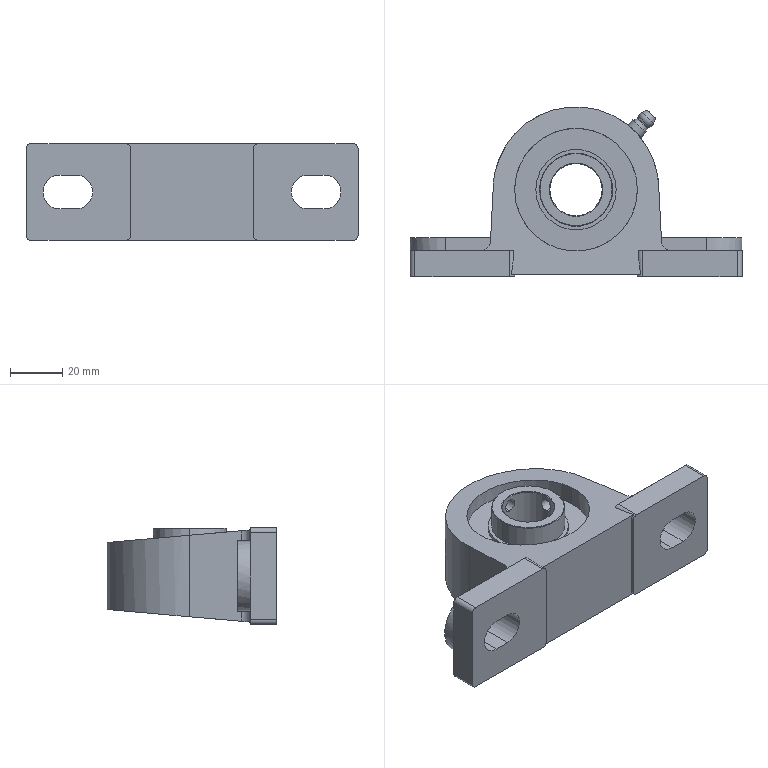Part | SolidWorks | features BaseBody 1 | 1 solid | 97 faces | box 127 x 65 x 37 mm | volume 115182 mm3 | cylinder 41 | plane 38 | cone 12 | torus 6 | commonest cylinder face diameters 3.7 x8 4.917 x4 7.4 x4 13 x4 28 x4 30.8 x4